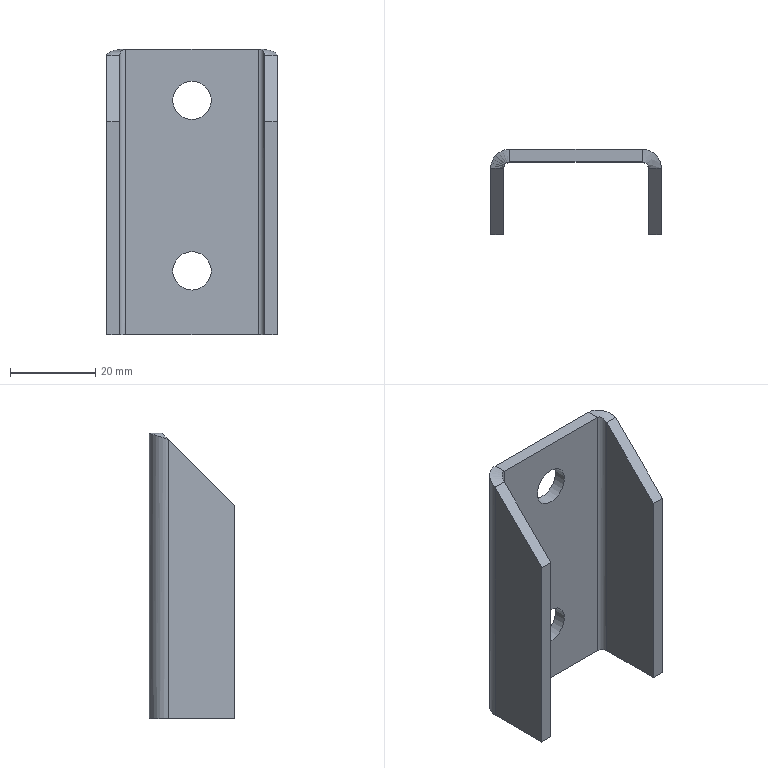Part | STEP file | 6100514 | 1 solid | 24 faces | box 40 x 20 x 67 mm | volume 13099 mm3 | plane 16 | cylinder 6 | spline 2 | commonest cylinder face diameters 9 x4 3 x2